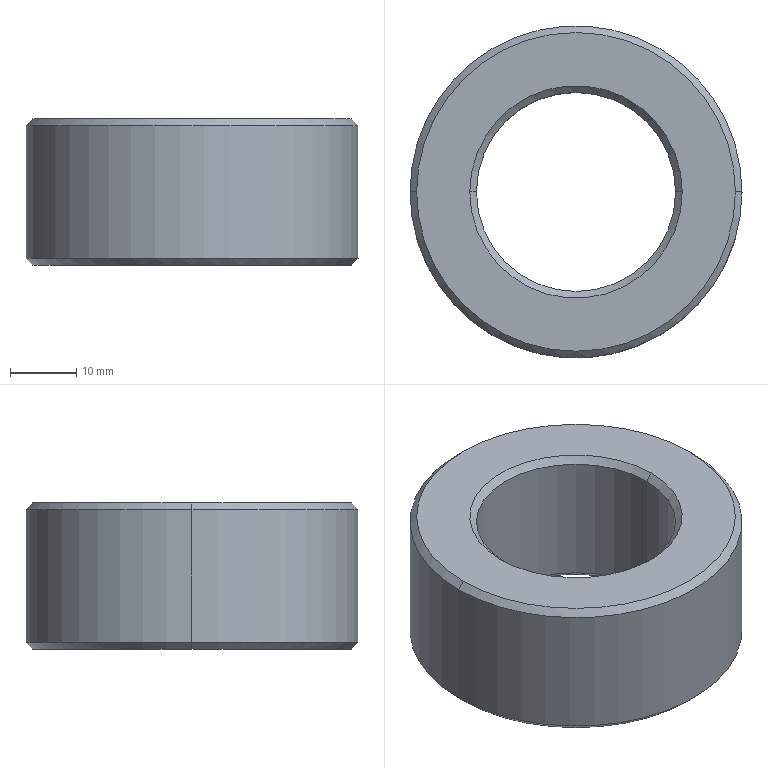Part | NX | features BREP 1 | 1 solid | 14 faces | box 50 x 50 x 22 mm | volume 27395 mm3 | cone 8 | cylinder 4 | plane 2 | commonest cylinder face diameters 30 x2 50 x2
STEP:
#1=CARTESIAN_POINT('',(15.,0.,21.));
#2=VERTEX_POINT('',#1);
#3=CARTESIAN_POINT('',(-15.,0.,21.));
#4=VERTEX_POINT('',#3);
#5=CARTESIAN_POINT('',(0.,0.,21.));
#6=DIRECTION('',(0.,0.,-1.));
#7=DIRECTION('',(1.,0.,0.));
#8=AXIS2_PLACEMENT_3D('',#5,#6,#7);
#9=CIRCLE('',#8,15.);
#10=EDGE_CURVE('',#2,#4,#9,.T.);
#11=ORIENTED_EDGE('',*,*,#10,.F.);
#12=CARTESIAN_POINT('',(15.,0.,1.));
#13=VERTEX_POINT('',#12);
#14=CARTESIAN_POINT('',(15.,0.,21.));
#15=DIRECTION('',(0.,0.,-1.));
#16=VECTOR('',#15,1000.);
#17=LINE('',#14,#16);
#18=EDGE_CURVE('',#13,#2,#17,.F.);
#19=ORIENTED_EDGE('',*,*,#18,.F.);
#20=CARTESIAN_POINT('',(-15.,0.,1.));
#21=VERTEX_POINT('',#20);
#22=CARTESIAN_POINT('',(0.,0.,1.));
#23=DIRECTION('',(0.,0.,1.));
#24=DIRECTION('',(0.5,-0.866,0.));
#25=AXIS2_PLACEMENT_3D('',#22,#23,#24);
#26=CIRCLE('',#25,15.);
#27=EDGE_CURVE('',#21,#13,#26,.T.);
#28=ORIENTED_EDGE('',*,*,#27,.F.);
#29=CARTESIAN_POINT('',(-15.,0.,21.));
#30=DIRECTION('',(0.,0.,-1.));
#31=VECTOR('',#30,1000.);
#32=LINE('',#29,#31);
#33=EDGE_CURVE('',#21,#4,#32,.F.);
#34=ORIENTED_EDGE('',*,*,#33,.T.);
#35=EDGE_LOOP('',(#11,#19,#28,#34));
#36=FACE_BOUND('',#35,.T.);
#37=CARTESIAN_POINT('',(0.,0.,11.));
#38=DIRECTION('',(0.,0.,1.));
#39=DIRECTION('',(1.,0.,0.));
#40=AXIS2_PLACEMENT_3D('',#37,#38,#39);
#41=CYLINDRICAL_SURFACE('',#40,15.);
#42=ADVANCED_FACE('',(#36),#41,.F.);
#43=CARTESIAN_POINT('',(16.,0.,22.));
#44=VERTEX_POINT('',#43);
#45=CARTESIAN_POINT('',(16.,0.,22.));
#46=DIRECTION('',(-0.7071,0.,-0.7071));
#47=VECTOR('',#46,1000.);
#48=LINE('',#45,#47);
#49=EDGE_CURVE('',#2,#44,#48,.F.);
#50=ORIENTED_EDGE('',*,*,#49,.F.);
#51=ORIENTED_EDGE('',*,*,#10,.T.);
#52=CARTESIAN_POINT('',(-16.,0.,22.));
#53=VERTEX_POINT('',#52);
#54=CARTESIAN_POINT('',(-16.,0.,22.));
#55=DIRECTION('',(0.7071,0.,-0.7071));
#56=VECTOR('',#55,1000.);
#57=LINE('',#54,#56);
#58=EDGE_CURVE('',#4,#53,#57,.F.);
#59=ORIENTED_EDGE('',*,*,#58,.T.);
#60=CARTESIAN_POINT('',(0.,0.,22.));
#61=DIRECTION('',(0.,0.,-1.));
#62=DIRECTION('',(0.5,-0.866,0.));
#63=AXIS2_PLACEMENT_3D('',#60,#61,#62);
#64=CIRCLE('',#63,16.);
#65=EDGE_CURVE('',#44,#53,#64,.T.);
#66=ORIENTED_EDGE('',*,*,#65,.F.);
#67=EDGE_LOOP('',(#50,#51,#59,#66));
#68=FACE_BOUND('',#67,.T.);
#69=CARTESIAN_POINT('',(0.,0.,21.5));
#70=DIRECTION('',(0.,0.,1.));
#71=DIRECTION('',(1.,0.,0.));
#72=AXIS2_PLACEMENT_3D('',#69,#70,#71);
#73=CONICAL_SURFACE('',#72,15.5,0.7854);
#74=ADVANCED_FACE('',(#68),#73,.F.);
#75=CARTESIAN_POINT('',(-24.,0.,22.));
#76=VERTEX_POINT('',#75);
#77=CARTESIAN_POINT('',(24.,0.,22.));
#78=VERTEX_POINT('',#77);
#79=CARTESIAN_POINT('',(0.,0.,22.));
#80=DIRECTION('',(0.,0.,1.));
#81=DIRECTION('',(-1.,0.,0.));
#82=AXIS2_PLACEMENT_3D('',#79,#80,#81);
#83=CIRCLE('',#82,24.);
#84=EDGE_CURVE('',#76,#78,#83,.T.);
#85=ORIENTED_EDGE('',*,*,#84,.T.);
#86=CARTESIAN_POINT('',(0.,0.,22.));
#87=DIRECTION('',(0.,0.,1.));
#88=DIRECTION('',(1.,0.,0.));
#89=AXIS2_PLACEMENT_3D('',#86,#87,#88);
#90=CIRCLE('',#89,24.);
#91=EDGE_CURVE('',#78,#76,#90,.T.);
#92=ORIENTED_EDGE('',*,*,#91,.T.);
#93=EDGE_LOOP('',(#85,#92));
#94=FACE_BOUND('',#93,.T.);
#95=CARTESIAN_POINT('',(0.,0.,22.));
#96=DIRECTION('',(0.,0.,-1.));
#97=DIRECTION('',(-1.,0.,0.));
#98=AXIS2_PLACEMENT_3D('',#95,#96,#97);
#99=CIRCLE('',#98,16.);
#100=EDGE_CURVE('',#53,#44,#99,.T.);
#101=ORIENTED_EDGE('',*,*,#100,.T.);
#102=ORIENTED_EDGE('',*,*,#65,.T.);
#103=EDGE_LOOP('',(#101,#102));
#104=FACE_BOUND('',#103,.T.);
#105=CARTESIAN_POINT('',(0.,0.,22.));
#106=DIRECTION('',(0.,0.,1.));
#107=DIRECTION('',(1.,0.,0.));
#108=AXIS2_PLACEMENT_3D('',#105,#106,#107);
#109=PLANE('',#108);
#110=ADVANCED_FACE('',(#94,#104),#109,.T.);
#111=CARTESIAN_POINT('',(25.,0.,21.));
#112=VERTEX_POINT('',#111);
#113=CARTESIAN_POINT('',(-25.,0.,21.));
#114=VERTEX_POINT('',#113);
#115=CARTESIAN_POINT('',(0.,0.,21.));
#116=DIRECTION('',(0.,0.,1.));
#117=DIRECTION('',(1.,0.,0.));
#118=AXIS2_PLACEMENT_3D('',#115,#116,#117);
#119=CIRCLE('',#118,25.);
#120=EDGE_CURVE('',#112,#114,#119,.T.);
#121=ORIENTED_EDGE('',*,*,#120,.T.);
#122=CARTESIAN_POINT('',(-24.,0.,22.));
#123=DIRECTION('',(-0.7071,0.,-0.7071));
#124=VECTOR('',#123,1000.);
#125=LINE('',#122,#124);
#126=EDGE_CURVE('',#76,#114,#125,.T.);
#127=ORIENTED_EDGE('',*,*,#126,.F.);
#128=ORIENTED_EDGE('',*,*,#91,.F.);
#129=CARTESIAN_POINT('',(25.,0.,21.));
#130=DIRECTION('',(-0.7071,0.,0.7071));
#131=VECTOR('',#130,1000.);
#132=LINE('',#129,#131);
#133=EDGE_CURVE('',#112,#78,#132,.T.);
#134=ORIENTED_EDGE('',*,*,#133,.F.);
#135=EDGE_LOOP('',(#121,#127,#128,#134));
#136=FACE_BOUND('',#135,.T.);
#137=CARTESIAN_POINT('',(0.,0.,21.5));
#138=DIRECTION('',(0.,0.,-1.));
#139=DIRECTION('',(1.,0.,0.));
#140=AXIS2_PLACEMENT_3D('',#137,#138,#139);
#141=CONICAL_SURFACE('',#140,24.5,0.7854);
#142=ADVANCED_FACE('',(#136),#141,.T.);
#143=ORIENTED_EDGE('',*,*,#126,.T.);
#144=CARTESIAN_POINT('',(0.,0.,21.));
#145=DIRECTION('',(0.,0.,1.));
#146=DIRECTION('',(-1.,0.,0.));
#147=AXIS2_PLACEMENT_3D('',#144,#145,#146);
#148=CIRCLE('',#147,25.);
#149=EDGE_CURVE('',#114,#112,#148,.T.);
#150=ORIENTED_EDGE('',*,*,#149,.T.);
#151=ORIENTED_EDGE('',*,*,#133,.T.);
#152=ORIENTED_EDGE('',*,*,#84,.F.);
#153=EDGE_LOOP('',(#143,#150,#151,#152));
#154=FACE_BOUND('',#153,.T.);
#155=CARTESIAN_POINT('',(0.,0.,21.5));
#156=DIRECTION('',(0.,0.,-1.));
#157=DIRECTION('',(1.,0.,0.));
#158=AXIS2_PLACEMENT_3D('',#155,#156,#157);
#159=CONICAL_SURFACE('',#158,24.5,0.7854);
#160=ADVANCED_FACE('',(#154),#159,.T.);
#161=CARTESIAN_POINT('',(25.,0.,1.));
#162=VERTEX_POINT('',#161);
#163=CARTESIAN_POINT('',(-25.,0.,1.));
#164=VERTEX_POINT('',#163);
#165=CARTESIAN_POINT('',(0.,0.,1.));
#166=DIRECTION('',(0.,0.,-1.));
#167=DIRECTION('',(0.5,-0.866,0.));
#168=AXIS2_PLACEMENT_3D('',#165,#166,#167);
#169=CIRCLE('',#168,25.);
#170=EDGE_CURVE('',#162,#164,#169,.T.);
#171=ORIENTED_EDGE('',*,*,#170,.F.);
#172=CARTESIAN_POINT('',(25.,0.,21.));
#173=DIRECTION('',(0.,0.,-1.));
#174=VECTOR('',#173,1000.);
#175=LINE('',#172,#174);
#176=EDGE_CURVE('',#162,#112,#175,.F.);
#177=ORIENTED_EDGE('',*,*,#176,.T.);
#178=ORIENTED_EDGE('',*,*,#149,.F.);
#179=CARTESIAN_POINT('',(-25.,0.,21.));
#180=DIRECTION('',(0.,0.,-1.));
#181=VECTOR('',#180,1000.);
#182=LINE('',#179,#181);
#183=EDGE_CURVE('',#164,#114,#182,.F.);
#184=ORIENTED_EDGE('',*,*,#183,.F.);
#185=EDGE_LOOP('',(#171,#177,#178,#184));
#186=FACE_BOUND('',#185,.T.);
#187=CARTESIAN_POINT('',(0.,0.,11.));
#188=DIRECTION('',(0.,0.,1.));
#189=DIRECTION('',(1.,0.,0.));
#190=AXIS2_PLACEMENT_3D('',#187,#188,#189);
#191=CYLINDRICAL_SURFACE('',#190,25.);
#192=ADVANCED_FACE('',(#186),#191,.T.);
#193=CARTESIAN_POINT('',(0.,0.,1.));
#194=DIRECTION('',(0.,0.,-1.));
#195=DIRECTION('',(-1.,0.,0.));
#196=AXIS2_PLACEMENT_3D('',#193,#194,#195);
#197=CIRCLE('',#196,25.);
#198=EDGE_CURVE('',#164,#162,#197,.T.);
#199=ORIENTED_EDGE('',*,*,#198,.F.);
#200=ORIENTED_EDGE('',*,*,#183,.T.);
#201=ORIENTED_EDGE('',*,*,#120,.F.);
#202=ORIENTED_EDGE('',*,*,#176,.F.);
#203=EDGE_LOOP('',(#199,#200,#201,#202));
#204=FACE_BOUND('',#203,.T.);
#205=CARTESIAN_POINT('',(0.,0.,11.));
#206=DIRECTION('',(0.,0.,1.));
#207=DIRECTION('',(1.,0.,0.));
#208=AXIS2_PLACEMENT_3D('',#205,#206,#207);
#209=CYLINDRICAL_SURFACE('',#208,25.);
#210=ADVANCED_FACE('',(#204),#209,.T.);
#211=CARTESIAN_POINT('',(-24.,0.,0.));
#212=VERTEX_POINT('',#211);
#213=CARTESIAN_POINT('',(24.,0.000000001,0.));
#214=VERTEX_POINT('',#213);
#215=CARTESIAN_POINT('',(0.,0.,0.));
#216=DIRECTION('',(0.,0.,-1.));
#217=DIRECTION('',(-1.,0.,0.));
#218=AXIS2_PLACEMENT_3D('',#215,#216,#217);
#219=CIRCLE('',#218,24.);
#220=EDGE_CURVE('',#212,#214,#219,.T.);
#221=ORIENTED_EDGE('',*,*,#220,.F.);
#222=CARTESIAN_POINT('',(-25.,0.,1.));
#223=DIRECTION('',(0.7071,0.,-0.7071));
#224=VECTOR('',#223,1000.);
#225=LINE('',#222,#224);
#226=EDGE_CURVE('',#164,#212,#225,.T.);
#227=ORIENTED_EDGE('',*,*,#226,.F.);
#228=ORIENTED_EDGE('',*,*,#198,.T.);
#229=CARTESIAN_POINT('',(25.,0.,1.));
#230=DIRECTION('',(-0.7071,0.,-0.7071));
#231=VECTOR('',#230,1000.);
#232=LINE('',#229,#231);
#233=EDGE_CURVE('',#162,#214,#232,.T.);
#234=ORIENTED_EDGE('',*,*,#233,.T.);
#235=EDGE_LOOP('',(#221,#227,#228,#234));
#236=FACE_BOUND('',#235,.T.);
#237=CARTESIAN_POINT('',(0.,0.,0.5));
#238=DIRECTION('',(0.,0.,1.));
#239=DIRECTION('',(1.,0.,0.));
#240=AXIS2_PLACEMENT_3D('',#237,#238,#239);
#241=CONICAL_SURFACE('',#240,24.5,0.7854);
#242=ADVANCED_FACE('',(#236),#241,.T.);
#243=ORIENTED_EDGE('',*,*,#233,.F.);
#244=ORIENTED_EDGE('',*,*,#170,.T.);
#245=ORIENTED_EDGE('',*,*,#226,.T.);
#246=CARTESIAN_POINT('',(0.,0.,0.));
#247=DIRECTION('',(0.,0.,-1.));
#248=DIRECTION('',(0.5,-0.866,0.));
#249=AXIS2_PLACEMENT_3D('',#246,#247,#248);
#250=CIRCLE('',#249,24.);
#251=EDGE_CURVE('',#214,#212,#250,.T.);
#252=ORIENTED_EDGE('',*,*,#251,.F.);
#253=EDGE_LOOP('',(#243,#244,#245,#252));
#254=FACE_BOUND('',#253,.T.);
#255=CARTESIAN_POINT('',(0.,0.,0.5));
#256=DIRECTION('',(0.,0.,1.));
#257=DIRECTION('',(1.,0.,0.));
#258=AXIS2_PLACEMENT_3D('',#255,#256,#257);
#259=CONICAL_SURFACE('',#258,24.5,0.7854);
#260=ADVANCED_FACE('',(#254),#259,.T.);
#261=ORIENTED_EDGE('',*,*,#251,.T.);
#262=ORIENTED_EDGE('',*,*,#220,.T.);
#263=EDGE_LOOP('',(#261,#262));
#264=FACE_BOUND('',#263,.T.);
#265=CARTESIAN_POINT('',(-16.,0.,0.));
#266=VERTEX_POINT('',#265);
#267=CARTESIAN_POINT('',(16.,0.,0.));
#268=VERTEX_POINT('',#267);
#269=CARTESIAN_POINT('',(0.,0.,0.));
#270=DIRECTION('',(0.,0.,1.));
#271=DIRECTION('',(0.5,-0.866,0.));
#272=AXIS2_PLACEMENT_3D('',#269,#270,#271);
#273=CIRCLE('',#272,16.);
#274=EDGE_CURVE('',#266,#268,#273,.T.);
#275=ORIENTED_EDGE('',*,*,#274,.T.);
#276=CARTESIAN_POINT('',(0.,0.,0.));
#277=DIRECTION('',(0.,0.,1.));
#278=DIRECTION('',(1.,0.,0.));
#279=AXIS2_PLACEMENT_3D('',#276,#277,#278);
#280=CIRCLE('',#279,16.);
#281=EDGE_CURVE('',#268,#266,#280,.T.);
#282=ORIENTED_EDGE('',*,*,#281,.T.);
#283=EDGE_LOOP('',(#275,#282));
#284=FACE_BOUND('',#283,.T.);
#285=CARTESIAN_POINT('',(0.,0.,0.));
#286=DIRECTION('',(0.,0.,1.));
#287=DIRECTION('',(1.,0.,0.));
#288=AXIS2_PLACEMENT_3D('',#285,#286,#287);
#289=PLANE('',#288);
#290=ADVANCED_FACE('',(#264,#284),#289,.F.);
#291=CARTESIAN_POINT('',(-15.,0.,1.));
#292=DIRECTION('',(-0.7071,0.,-0.7071));
#293=VECTOR('',#292,1000.);
#294=LINE('',#291,#293);
#295=EDGE_CURVE('',#21,#266,#294,.T.);
#296=ORIENTED_EDGE('',*,*,#295,.F.);
#297=ORIENTED_EDGE('',*,*,#27,.T.);
#298=CARTESIAN_POINT('',(16.,0.,0.));
#299=DIRECTION('',(-0.7071,0.,0.7071));
#300=VECTOR('',#299,1000.);
#301=LINE('',#298,#300);
#302=EDGE_CURVE('',#268,#13,#301,.T.);
#303=ORIENTED_EDGE('',*,*,#302,.F.);
#304=ORIENTED_EDGE('',*,*,#274,.F.);
#305=EDGE_LOOP('',(#296,#297,#303,#304));
#306=FACE_BOUND('',#305,.T.);
#307=CARTESIAN_POINT('',(0.,0.,0.5));
#308=DIRECTION('',(0.,0.,-1.));
#309=DIRECTION('',(1.,0.,0.));
#310=AXIS2_PLACEMENT_3D('',#307,#308,#309);
#311=CONICAL_SURFACE('',#310,15.5,0.7854);
#312=ADVANCED_FACE('',(#306),#311,.F.);
#313=CARTESIAN_POINT('',(0.,0.,1.));
#314=DIRECTION('',(0.,0.,1.));
#315=DIRECTION('',(1.,0.,0.));
#316=AXIS2_PLACEMENT_3D('',#313,#314,#315);
#317=CIRCLE('',#316,15.);
#318=EDGE_CURVE('',#13,#21,#317,.T.);
#319=ORIENTED_EDGE('',*,*,#318,.T.);
#320=ORIENTED_EDGE('',*,*,#295,.T.);
#321=ORIENTED_EDGE('',*,*,#281,.F.);
#322=ORIENTED_EDGE('',*,*,#302,.T.);
#323=EDGE_LOOP('',(#319,#320,#321,#322));
#324=FACE_BOUND('',#323,.T.);
#325=CARTESIAN_POINT('',(0.,0.,0.5));
#326=DIRECTION('',(0.,0.,-1.));
#327=DIRECTION('',(1.,0.,0.));
#328=AXIS2_PLACEMENT_3D('',#325,#326,#327);
#329=CONICAL_SURFACE('',#328,15.5,0.7854);
#330=ADVANCED_FACE('',(#324),#329,.F.);
#331=ORIENTED_EDGE('',*,*,#33,.F.);
#332=ORIENTED_EDGE('',*,*,#318,.F.);
#333=ORIENTED_EDGE('',*,*,#18,.T.);
#334=CARTESIAN_POINT('',(0.,0.,21.));
#335=DIRECTION('',(0.,0.,-1.));
#336=DIRECTION('',(-1.,0.,0.));
#337=AXIS2_PLACEMENT_3D('',#334,#335,#336);
#338=CIRCLE('',#337,15.);
#339=EDGE_CURVE('',#4,#2,#338,.T.);
#340=ORIENTED_EDGE('',*,*,#339,.F.);
#341=EDGE_LOOP('',(#331,#332,#333,#340));
#342=FACE_BOUND('',#341,.T.);
#343=CARTESIAN_POINT('',(0.,0.,11.));
#344=DIRECTION('',(0.,0.,1.));
#345=DIRECTION('',(1.,0.,0.));
#346=AXIS2_PLACEMENT_3D('',#343,#344,#345);
#347=CYLINDRICAL_SURFACE('',#346,15.);
#348=ADVANCED_FACE('',(#342),#347,.F.);
#349=ORIENTED_EDGE('',*,*,#100,.F.);
#350=ORIENTED_EDGE('',*,*,#58,.F.);
#351=ORIENTED_EDGE('',*,*,#339,.T.);
#352=ORIENTED_EDGE('',*,*,#49,.T.);
#353=EDGE_LOOP('',(#349,#350,#351,#352));
#354=FACE_BOUND('',#353,.T.);
#355=CARTESIAN_POINT('',(0.,0.,21.5));
#356=DIRECTION('',(0.,0.,1.));
#357=DIRECTION('',(1.,0.,0.));
#358=AXIS2_PLACEMENT_3D('',#355,#356,#357);
#359=CONICAL_SURFACE('',#358,15.5,0.7854);
#360=ADVANCED_FACE('',(#354),#359,.F.);
#361=CLOSED_SHELL('',(#42,#74,#110,#142,#160,#192,#210,#242,#260,#290,#312,#330,#348,#360));
#362=MANIFOLD_SOLID_BREP('',#361);
#363=(LENGTH_UNIT()NAMED_UNIT(*)SI_UNIT(.MILLI.,.METRE.));
#364=UNCERTAINTY_MEASURE_WITH_UNIT(LENGTH_MEASURE(0.00001),#363,'','');
#365=(NAMED_UNIT(*)PLANE_ANGLE_UNIT()SI_UNIT($,.RADIAN.));
#366=(NAMED_UNIT(*)SI_UNIT($,.STERADIAN.)SOLID_ANGLE_UNIT());
#367=(GEOMETRIC_REPRESENTATION_CONTEXT(3)GLOBAL_UNCERTAINTY_ASSIGNED_CONTEXT((#364))GLOBAL_UNIT_ASSIGNED_CONTEXT((#363,#365,#366))REPRESENTATION_CONTEXT('',''));
#368=ADVANCED_BREP_SHAPE_REPRESENTATION('',(#362),#367);